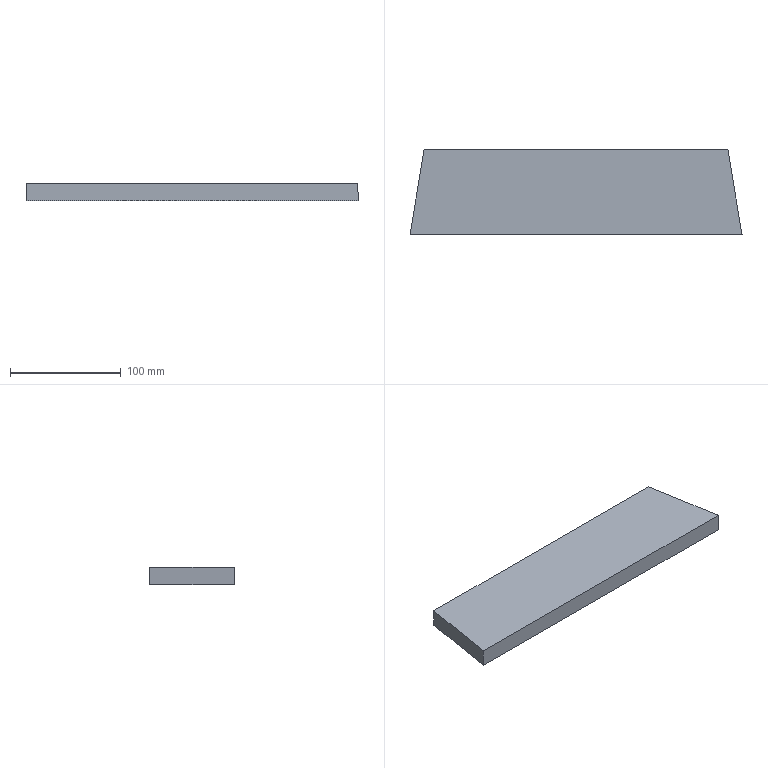Part | SolidWorks | features BaseBody 1 | 1 solid | 6 faces | box 300.429 x 76.2 x 16 mm | volume 350736 mm3 | plane 6
STEP:
#1=CARTESIAN_POINT('',(194.187,65.91,0.));
#2=VERTEX_POINT('',#1);
#3=CARTESIAN_POINT('',(-80.738,65.91,0.));
#4=VERTEX_POINT('',#3);
#5=CARTESIAN_POINT('',(56.724,65.91,0.));
#6=DIRECTION('',(-1.,0.,0.));
#7=VECTOR('',#6,1000.);
#8=LINE('',#5,#7);
#9=EDGE_CURVE('',#2,#4,#8,.T.);
#10=ORIENTED_EDGE('',*,*,#9,.F.);
#11=CARTESIAN_POINT('',(206.939,-10.29,0.));
#12=VERTEX_POINT('',#11);
#13=CARTESIAN_POINT('',(206.939,-10.29,0.));
#14=DIRECTION('',(-0.165,0.9863,0.));
#15=VECTOR('',#14,1000.);
#16=LINE('',#13,#15);
#17=EDGE_CURVE('',#12,#2,#16,.T.);
#18=ORIENTED_EDGE('',*,*,#17,.F.);
#19=CARTESIAN_POINT('',(-93.49,-10.29,0.));
#20=VERTEX_POINT('',#19);
#21=CARTESIAN_POINT('',(56.724,-10.29,0.));
#22=DIRECTION('',(1.,0.,0.));
#23=VECTOR('',#22,1000.);
#24=LINE('',#21,#23);
#25=EDGE_CURVE('',#20,#12,#24,.T.);
#26=ORIENTED_EDGE('',*,*,#25,.F.);
#27=CARTESIAN_POINT('',(-80.738,65.91,0.));
#28=DIRECTION('',(-0.165,-0.9863,0.));
#29=VECTOR('',#28,1000.);
#30=LINE('',#27,#29);
#31=EDGE_CURVE('',#4,#20,#30,.T.);
#32=ORIENTED_EDGE('',*,*,#31,.F.);
#33=EDGE_LOOP('',(#10,#18,#26,#32));
#34=FACE_OUTER_BOUND('',#33,.T.);
#35=CARTESIAN_POINT('',(56.724,26.478,0.));
#36=DIRECTION('',(0.,0.,1.));
#37=DIRECTION('',(1.,0.,0.));
#38=AXIS2_PLACEMENT_3D('',#35,#36,#37);
#39=PLANE('',#38);
#40=ADVANCED_FACE('',(#34),#39,.F.);
#41=ORIENTED_EDGE('',*,*,#31,.T.);
#42=CARTESIAN_POINT('',(-93.49,-10.29,16.));
#43=VERTEX_POINT('',#42);
#44=CARTESIAN_POINT('',(-93.49,-10.29,0.));
#45=DIRECTION('',(0.,0.,1.));
#46=VECTOR('',#45,1000.);
#47=LINE('',#44,#46);
#48=EDGE_CURVE('',#20,#43,#47,.T.);
#49=ORIENTED_EDGE('',*,*,#48,.T.);
#50=CARTESIAN_POINT('',(-80.738,65.91,16.));
#51=VERTEX_POINT('',#50);
#52=CARTESIAN_POINT('',(-93.49,-10.29,16.));
#53=DIRECTION('',(0.165,0.9863,0.));
#54=VECTOR('',#53,1000.);
#55=LINE('',#52,#54);
#56=EDGE_CURVE('',#43,#51,#55,.T.);
#57=ORIENTED_EDGE('',*,*,#56,.T.);
#58=CARTESIAN_POINT('',(-80.738,65.91,0.));
#59=DIRECTION('',(0.,0.,-1.));
#60=VECTOR('',#59,1000.);
#61=LINE('',#58,#60);
#62=EDGE_CURVE('',#51,#4,#61,.T.);
#63=ORIENTED_EDGE('',*,*,#62,.T.);
#64=EDGE_LOOP('',(#41,#49,#57,#63));
#65=FACE_OUTER_BOUND('',#64,.T.);
#66=CARTESIAN_POINT('',(-93.49,-10.29,0.));
#67=DIRECTION('',(-0.9863,0.165,0.));
#68=DIRECTION('',(-0.165,-0.9863,0.));
#69=AXIS2_PLACEMENT_3D('',#66,#67,#68);
#70=PLANE('',#69);
#71=ADVANCED_FACE('',(#65),#70,.T.);
#72=ORIENTED_EDGE('',*,*,#9,.T.);
#73=ORIENTED_EDGE('',*,*,#62,.F.);
#74=CARTESIAN_POINT('',(194.187,65.91,16.));
#75=VERTEX_POINT('',#74);
#76=CARTESIAN_POINT('',(-80.738,65.91,16.));
#77=DIRECTION('',(1.,0.,0.));
#78=VECTOR('',#77,1000.);
#79=LINE('',#76,#78);
#80=EDGE_CURVE('',#51,#75,#79,.T.);
#81=ORIENTED_EDGE('',*,*,#80,.T.);
#82=CARTESIAN_POINT('',(194.187,65.91,0.));
#83=DIRECTION('',(0.,0.,-1.));
#84=VECTOR('',#83,1000.);
#85=LINE('',#82,#84);
#86=EDGE_CURVE('',#75,#2,#85,.T.);
#87=ORIENTED_EDGE('',*,*,#86,.T.);
#88=EDGE_LOOP('',(#72,#73,#81,#87));
#89=FACE_OUTER_BOUND('',#88,.T.);
#90=CARTESIAN_POINT('',(-80.738,65.91,0.));
#91=DIRECTION('',(0.,1.,0.));
#92=DIRECTION('',(0.,0.,1.));
#93=AXIS2_PLACEMENT_3D('',#90,#91,#92);
#94=PLANE('',#93);
#95=ADVANCED_FACE('',(#89),#94,.T.);
#96=ORIENTED_EDGE('',*,*,#17,.T.);
#97=ORIENTED_EDGE('',*,*,#86,.F.);
#98=CARTESIAN_POINT('',(206.939,-10.29,16.));
#99=VERTEX_POINT('',#98);
#100=CARTESIAN_POINT('',(194.187,65.91,16.));
#101=DIRECTION('',(0.165,-0.9863,0.));
#102=VECTOR('',#101,1000.);
#103=LINE('',#100,#102);
#104=EDGE_CURVE('',#75,#99,#103,.T.);
#105=ORIENTED_EDGE('',*,*,#104,.T.);
#106=CARTESIAN_POINT('',(206.939,-10.29,0.));
#107=DIRECTION('',(0.,0.,-1.));
#108=VECTOR('',#107,1000.);
#109=LINE('',#106,#108);
#110=EDGE_CURVE('',#99,#12,#109,.T.);
#111=ORIENTED_EDGE('',*,*,#110,.T.);
#112=EDGE_LOOP('',(#96,#97,#105,#111));
#113=FACE_OUTER_BOUND('',#112,.T.);
#114=CARTESIAN_POINT('',(194.187,65.91,0.));
#115=DIRECTION('',(0.9863,0.165,0.));
#116=DIRECTION('',(-0.165,0.9863,0.));
#117=AXIS2_PLACEMENT_3D('',#114,#115,#116);
#118=PLANE('',#117);
#119=ADVANCED_FACE('',(#113),#118,.T.);
#120=ORIENTED_EDGE('',*,*,#25,.T.);
#121=ORIENTED_EDGE('',*,*,#110,.F.);
#122=CARTESIAN_POINT('',(206.939,-10.29,16.));
#123=DIRECTION('',(-1.,0.,0.));
#124=VECTOR('',#123,1000.);
#125=LINE('',#122,#124);
#126=EDGE_CURVE('',#99,#43,#125,.T.);
#127=ORIENTED_EDGE('',*,*,#126,.T.);
#128=ORIENTED_EDGE('',*,*,#48,.F.);
#129=EDGE_LOOP('',(#120,#121,#127,#128));
#130=FACE_OUTER_BOUND('',#129,.T.);
#131=CARTESIAN_POINT('',(206.939,-10.29,0.));
#132=DIRECTION('',(0.,-1.,0.));
#133=DIRECTION('',(1.,0.,0.));
#134=AXIS2_PLACEMENT_3D('',#131,#132,#133);
#135=PLANE('',#134);
#136=ADVANCED_FACE('',(#130),#135,.T.);
#137=ORIENTED_EDGE('',*,*,#126,.F.);
#138=ORIENTED_EDGE('',*,*,#104,.F.);
#139=ORIENTED_EDGE('',*,*,#80,.F.);
#140=ORIENTED_EDGE('',*,*,#56,.F.);
#141=EDGE_LOOP('',(#137,#138,#139,#140));
#142=FACE_OUTER_BOUND('',#141,.T.);
#143=CARTESIAN_POINT('',(56.724,26.478,16.));
#144=DIRECTION('',(0.,0.,1.));
#145=DIRECTION('',(1.,0.,0.));
#146=AXIS2_PLACEMENT_3D('',#143,#144,#145);
#147=PLANE('',#146);
#148=ADVANCED_FACE('',(#142),#147,.T.);
#149=CLOSED_SHELL('',(#40,#71,#95,#119,#136,#148));
#150=MANIFOLD_SOLID_BREP('',#149);
#151=CARTESIAN_POINT('',(0.,0.,0.));
#152=DIRECTION('',(0.,0.,1.));
#153=DIRECTION('',(1.,0.,0.));
#154=AXIS2_PLACEMENT_3D('',#151,#152,#153);
#155=(LENGTH_UNIT()NAMED_UNIT(*)SI_UNIT(.MILLI.,.METRE.));
#156=UNCERTAINTY_MEASURE_WITH_UNIT(LENGTH_MEASURE(0.00001),#155,'','');
#157=(NAMED_UNIT(*)PLANE_ANGLE_UNIT()SI_UNIT($,.RADIAN.));
#158=(NAMED_UNIT(*)SI_UNIT($,.STERADIAN.)SOLID_ANGLE_UNIT());
#159=(GEOMETRIC_REPRESENTATION_CONTEXT(3)GLOBAL_UNCERTAINTY_ASSIGNED_CONTEXT((#156))GLOBAL_UNIT_ASSIGNED_CONTEXT((#155,#157,#158))REPRESENTATION_CONTEXT('',''));
#160=ADVANCED_BREP_SHAPE_REPRESENTATION('',(#150,#154),#159);